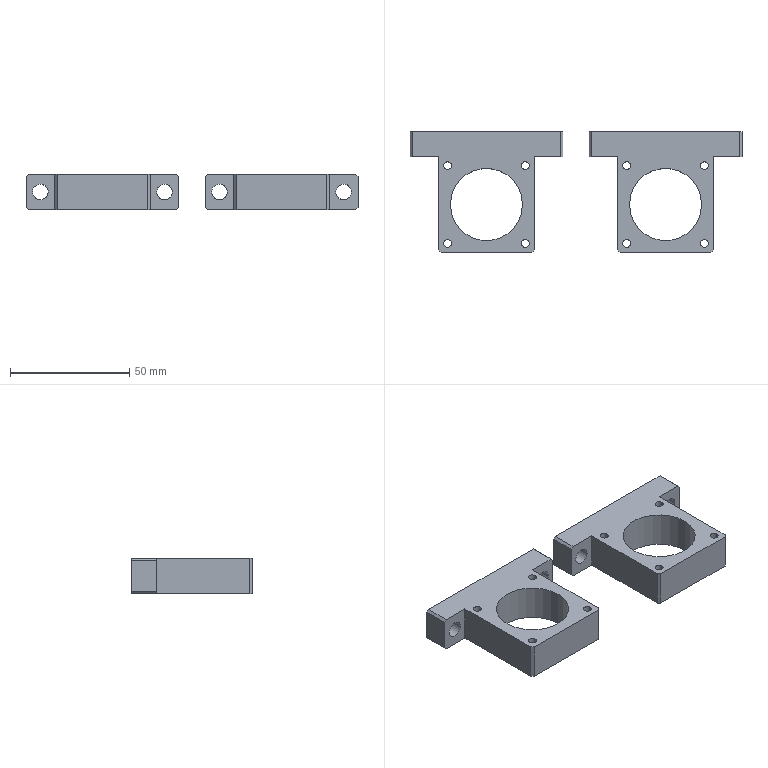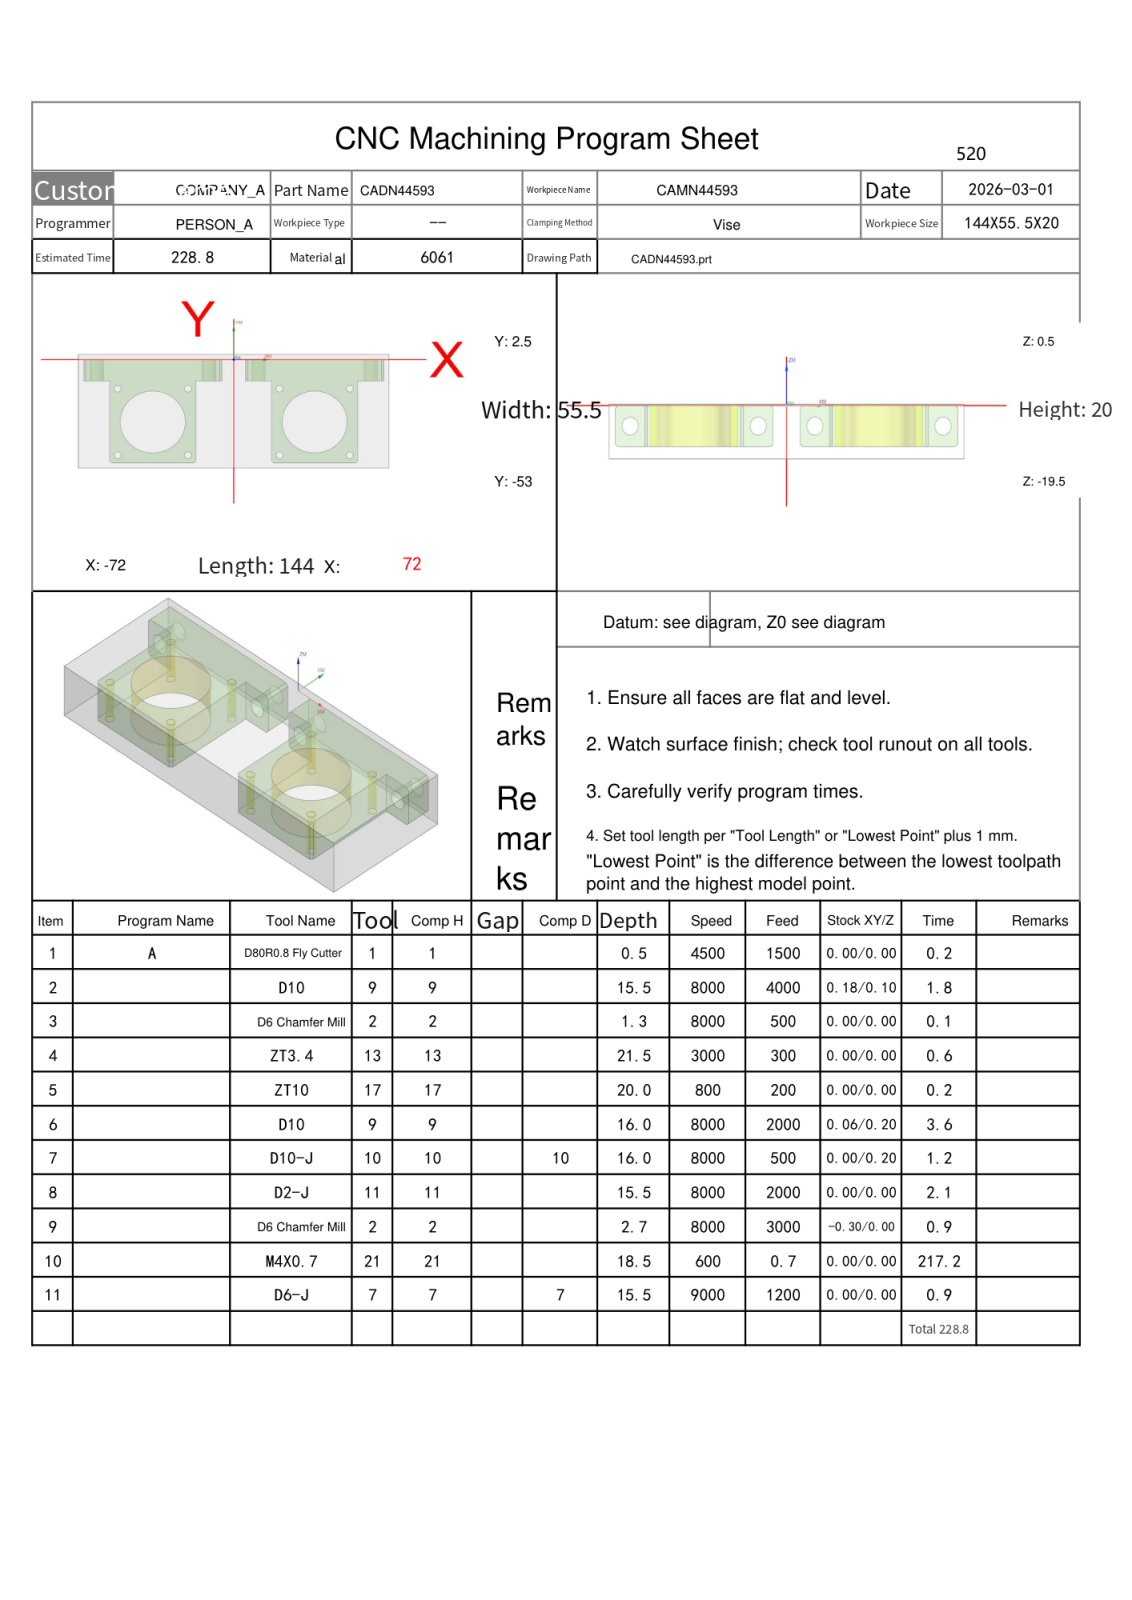NC program | NX | posted by the shop | part box 139 x 50.5 x 15 mm
Lines 36 to 892 of 10033:
N2 T09 M06
(D10  D=10. R=0. H=09 ce=0.25 di=0.10)
G00 G90 G54 X-82.431 Y-11.514 M03 S8000
G43 H09 Z50.
M08
Z-13.
G01 X-82.332 Y-11.496 Z-13.625 F4000.
X-82.234 Y-11.477 Z-13.872
X-82.136 Y-11.458 Z-14.054
X-82.038 Y-11.44 Z-14.2
X-81.939 Y-11.421 Z-14.323
X-81.841 Y-11.402 Z-14.428
X-81.743 Y-11.384 Z-14.52
X-81.645 Y-11.365 Z-14.6
X-81.546 Y-11.346 Z-14.67
X-81.448 Y-11.328 Z-14.732
X-81.35 Y-11.309 Z-14.786
X-81.252 Y-11.29 Z-14.833
X-81.153 Y-11.272 Z-14.874
X-81.055 Y-11.253 Z-14.908
X-80.957 Y-11.234 Z-14.936
X-80.859 Y-11.216 Z-14.96
X-80.761 Y-11.197 Z-14.977
X-80.662 Y-11.178 Z-14.99
X-80.564 Y-11.16 Z-14.997
X-80.466 Y-11.141 Z-15.
X-78.352 Y-10.739
G03 X-78. Y-10.48 I-.101 J.505
X-77.362 Y-6.666 I-12.273 J4.014
X-77.171 Y.847 I-456.093 J15.32
G02 X-73.96 Y5.724 I6.172 J-.569
X-68.324 Y7.378 I6.632 J-12.167
X-60.544 Y7.699 I7.779 J-93.942
X-59.293 Y7.691 I0.0 J-94.264
G01 X70.13 Y7.678
G02 X75.219 Y4.452 I-.351 J-6.181
X76.887 Y-1.277 I-12.247 J-6.672
X77.2 Y-9.063 I-96.712 J-7.786
X77.192 Y-10.308 I-97.025 J0.0
G01 X77.178 Y-51.13
G02 X73.969 Y-56.209 I-6.178 J.35
X68.412 Y-57.866 I-6.606 J12.012
X60.704 Y-58.198 I-7.708 J89.284
X59.542 Y-58.19 I0.0 J89.616
G01 X-70.15 Y-58.176
G02 X-75.222 Y-54.947 I.374 J6.185
X-76.868 Y-49.389 I12.074 J6.599
X-77.206 Y-41.288 I97.034 J8.1
X-77.193 Y-39.718 I97.372 J0.0
G01 X-77.183 Y-13.259
G03 X-76.595 Y-6.386 I-443.932 J41.454
G02 X-76.388 Y-1.091 I468.298 J-15.653
X-72.222 Y4.757 I7.74 J-1.105
X-65.87 Y6.544 I7.573 J-14.737
X-57.126 Y6.901 I8.744 J-106.812
X-55.64 Y6.891 I0.0 J-107.17
G01 X67.987 Y6.879
G02 X74.202 Y2.785 I-.602 J-7.679
X76.033 Y-3.55 I-14.344 J-7.577
X76.402 Y-12.347 I-104.524 J-8.797
X76.391 Y-13.859 I-104.894 J0.0
G01 X76.379 Y-48.987
G02 X72.413 Y-55.125 I-7.648 J.591
X66.168 Y-57.003 I-7.584 J13.897
X57.695 Y-57.396 I-8.473 J91.309
X56.5 Y-57.388 I0.0 J91.702
G01 X-67.987 Y-57.379
G02 X-74.125 Y-53.413 I.591 J7.648
X-76.003 Y-47.168 I13.895 J7.585
X-76.395 Y-38.7 I91.242 J8.468
X-76.388 Y-37.5 I91.635 J0.0
G01 X-76.379 Y-14.881
G02 X-75.807 Y-6.094 I948.959 J-57.37
X-75.532 Y-2.233 I27.725 J-.031
X-74.749 Y.011 I10.239 J-2.318
G01 X-74.571 Y1.359
X-74.047 Y2.625
X-73.212 Y3.712
X-72.125 Y4.547
X-70.859 Y5.071
G02 X-57.018 Y6.08 I13.841 J-94.414
X-56.024 Y6.075 I0.0 J-95.423
G01 X65.955 Y6.076
G02 X69.277 Y5.268 I-.437 J-9.032
G01 X70.859 Y5.071
X72.125 Y4.547
X73.212 Y3.712
X74.047 Y2.625
X74.571 Y1.359
G02 X75.577 Y-12.39 I-93.437 J-13.748
G01 X75.576 Y-12.82
X75.575 Y-46.959
G02 X70.823 Y-54.292 I-8.747 J.463
X64.171 Y-56.187 I-8.15 J15.986
X54.605 Y-56.608 I-9.566 J108.501
X52.744 Y-56.592 I0.0 J108.921
G01 X-65.956 Y-56.575
G02 X-73.291 Y-51.823 I.46 J8.748
X-75.177 Y-45.251 I15.886 J8.116
X-75.593 Y-36.287 I96.443 J8.963
X-75.586 Y-35.104 I96.859 J0.0
X-75.621 Y-26.982 I943.081 J8.122
X-75.546 Y-15.125 I943.116 J0.0
X-74.908 Y-4.653 I566.659 J-29.296
G01 X-74.75 Y-3.687
X-74.739 Y.081
G02 X-74.733 Y-2.973 I-765.948 J-3.054
X-74.784 Y-11.75 I-765.954 J0.0
G03 X-74.978 Y-23.864 I376.811 J-12.114
X-74.958 Y-27.735 I377.006 J0.0
X-74.977 Y-30.988 I290.447 J-3.254
X-74.769 Y-41.972 I290.465 J0.0
X-73.565 Y-49.046 I25.763 J.744
X-66.385 Y-55.337 I8.769 J2.765
X-59.903 Y-55.919 I6.482 J35.854
X-59.54 Y-55.917 I0.0 J36.435
G01 X-48.821 Y-55.958
X55.639 Y-55.931
G03 X56.143 Y-55.933 I.504 J68.081
X64.577 Y-55.409 I0.0 J68.083
X70.57 Y-53.308 I-1.709 J14.474
X74.323 Y-47.452 I-5.219 J7.475
X74.925 Y-40.804 I-36.403 J6.648
X74.921 Y-40.289 I-37.005 J0.0
G01 X74.958 Y-21.509
G03 X74.974 Y-18.479 I-302.812 J3.03
X74.75 Y-6.843 I-302.827 J0.0
G01 Y-.002
Y-10.502
G03 X74.175 Y-18.196 I51.208 J-7.694
X74.182 Y-19.024 I51.783 J0.0
G01 X74.119 Y-39.688
G02 X74.121 Y-40.113 I-33.926 J-.425
X73.539 Y-46.371 I-33.929 J0.0
X67.783 Y-53.21 I-9.493 J2.149
X60.803 Y-54.831 I-8.326 J20.008
G03 X59.177 Y-55.005 I.063 J-8.269
G02 X56.639 Y-55.748 I-2.829 J4.959
G01 X18.498 Y-55.75
G03 X10.852 Y-55.183 I-7.646 J-51.258
X10.208 Y-55.187 I0.0 J-51.826
G01 X-16.148 Y-55.171
X-17.141 Y-55.571
X-18.502 Y-55.75
X-56.642 Y-55.748
G03 X-63.405 Y-54.926 I-17.06 J-112.182
G02 X-68.664 Y-53.161 I.998 J11.687
X-72.813 Y-47.233 I6.532 J8.988
X-73.982 Y-39.664 I28.771 J8.321
X-74.182 Y-26.992 I402.551 J12.671
X-74.156 Y-22.466 I402.75 J0.0
X-74.05 Y-13.132 I612.773 J-2.32
G01 X-74.571 Y-11.859
X-74.75 Y-10.5
X-74.571 Y-11.859
G02 X-73.631 Y-15.867 I-8.072 J-4.008
G01 Y-15.908
G02 X-73.493 Y-26.765 I-426.487 J-10.858
X-73.51 Y-30.613 I-426.625 J0.0
G03 X-73.52 Y-32.179 I120.675 J-1.566
X-73.149 Y-41.643 I120.685 J0.0
X-71.428 Y-48.35 I19.187 J1.348
X-64.936 Y-53.583 I9.13 J4.683
X-59.767 Y-54.635 I11.418 J42.874
X-57.879 Y-55.57 I4.27 J6.245
G02 X-59.94 Y-54.497 I2.18 J6.698
G03 X-63.341 Y-53.256 I-10.094 J-22.38
G02 X-69.204 Y-49.355 I3.288 J11.298
X-71.958 Y-42.678 I12.418 J9.029
X-72.663 Y-33.723 I56.485 J8.955
G01 Y-33.515
X-72.775 Y-18.171
Y-18.061
G03 X-73.149 Y-14.317 I-18.885 J0.0
G01 X-74.047 Y-13.125
G02 X-72.957 Y-14.636 I-7.181 J-6.325
X-72.241 Y-18.739 I-12.6 J-4.313
X-72.046 Y-29.331 I-287.569 J-10.592
X-72.051 Y-31.028 I-287.764 J0.0
G03 X-72.056 Y-31.857 I74.824 J-.83
X-71.475 Y-41.163 I74.828 J0.0
X-69.154 Y-47.762 I16.108 J1.957
X-63.631 Y-52.166 I10.343 J7.308
G02 X-61.112 Y-53.319 I-20.619 J-48.377
G03 X-59.669 Y-54.684 I28.432 J28.599
G02 X-61.112 Y-53.319 I10.189 J12.211
G03 X-63.344 Y-51.644 I-7.49 J-7.657
G02 X-68.751 Y-46.08 I7.259 J12.463
X-70.803 Y-38.723 I18.983 J9.261
X-71.27 Y-28.82 I104.897 J9.903
X-71.265 Y-27.778 I105.364 J0.0
G03 X-71.256 Y-26.385 I-114.303 J1.393
X-71.552 Y-18.17 I-114.312 J0.0
X-72.325 Y-14.916 I-9.237 J-.477
G01 X-73.212 Y-14.212
G02 X-72.137 Y-15.11 I-2.708 J-4.339
X-71.08 Y-18.419 I-7.003 J-4.061
X-70.656 Y-25.71 I-62.477 J-7.291
G01 Y-25.957
X-70.657 Y-26.409
G03 X-70.267 Y-37.215 I149.848 J0.0
X-68.421 Y-44.795 I22.579 J1.482
X-63.647 Y-50.425 I13.848 J6.904
G02 X-62.356 Y-51.504 I-5.852 J-8.313
G03 X-61.225 Y-53.196 I5.165 J2.23
G02 X-62.473 Y-51.245 I4.692 J4.377
G03 X-64.739 Y-48.532 I-23.525 J-17.349
G02 X-69.063 Y-38.943 I14.543 J12.327
X-69.794 Y-28.991 I67.41 J9.952
G01 Y-28.979
Y-28.838
G03 X-70.193 Y-19.713 I-104.458 J0.0
X-71.268 Y-15.662 I-11.361 J-.847
X-72.125 Y-15.047 I-1.109 J-.64
G01 X-72.379 Y-14.852
G03 X-71.53 Y-15.293 I1.458 J1.768
G02 X-70.22 Y-17.527 I-3.011 J-3.268
X-69.36 Y-23.349 I-23.843 J-6.496
G03 X-68.953 Y-33.765 I924.383 J30.898
X-67.431 Y-42.243 I31.323 J1.249
X-63.91 Y-48.305 I19.584 J7.322
G02 X-62.711 Y-49.98 I-10.07 J-8.467
G03 X-62.344 Y-51.499 I4.612 J.312
G02 X-62.758 Y-49.691 I6.886 J2.53
G03 X-64.405 Y-46.484 I-17.564 J-6.992
G02 X-67.928 Y-35.183 I23.689 J13.585
X-68.496 Y-24.9 I170.445 J14.57
G03 X-69.37 Y-18.191 I-30.901 J-.615
X-70.631 Y-15.67 I-5.904 J-1.377
G01 X-71.598 Y-15.265
G02 X-70.51 Y-15.718 I-2.748 J-8.132
X-68.968 Y-18.253 I-3.654 J-3.959
X-67.945 Y-24.45 I-24.694 J-7.259
G03 X-67.341 Y-34.242 I316.925 J14.627
X-63.573 Y-46.518 I29.872 J2.452
G02 X-62.75 Y-48.355 I-12.898 J-6.884
G01 X-62.751 Y-48.562
G03 X-62.708 Y-49.917 I21.649 J0.0
G02 X-62.762 Y-47.989 I34.497 J1.928
G01 Y-47.948
G03 X-63.736 Y-44.797 I-14.136 J-2.643
G02 X-66.704 Y-31.486 I37.919 J15.44
G03 X-67.39 Y-22.37 I-180.615 J-9.014
X-68.834 Y-17.111 I-15.436 J-1.412
X-70.058 Y-15.686 I-2.961 J-1.306
G01 X-70.859 Y-15.571
G02 X-69.766 Y-15.79 I-.065 J-3.162
X-67.969 Y-18.171 I-2.941 J-4.088
X-66.629 Y-24.212 I-19.916 J-7.587
G03 X-65.835 Y-33.62 I890.373 J70.394
X-63.21 Y-44.292 I43.374 J5.012
G01 X-62.75 Y-45.743
Y-48.143
G03 X-62.727 Y-46.823 I-37.301 J1.32
X-62.798 Y-44.518 I-37.325 J0.0
X-63.99 Y-39.239 I-75.218 J-14.218
G02 X-65.465 Y-28.379 I71.773 J15.276
G03 X-66.515 Y-20.531 I-49.341 J-2.608
X-68.472 Y-16.358 I-9.618 J-1.964
X-69.322 Y-15.75 I-1.342 J-.979
G01 X-70.057 Y-15.677
G02 X-68.974 Y-15.829 I-.159 J-5.043
X-66.967 Y-18.096 I-2.488 J-4.224
X-65.33 Y-24.057 I-17.553 J-8.026
X-64.328 Y-33.318 I-746.439 J-85.447
G03 X-62.75 Y-41.617 I79.908 J10.89
G01 Y-45.057
G03 X-62.727 Y-42.921 I-100.07 J2.136
X-62.798 Y-39.166 I-100.093 J0.0
G02 X-64.402 Y-25.217 I930.073 J114.005
G03 X-66.051 Y-18.619 I-23.568 J-2.389
X-68.259 Y-15.82 I-5.837 J-2.331
X-68.975 Y-15.732 I-.716 J-2.882
X-69.298 Y-15.75 I0.0 J-2.97
G02 X-68.929 Y-15.73 I.369 J-3.387
X-68.13 Y-15.825 I0.0 J-3.407
X-65.914 Y-18.081 I-2.318 J-4.493
X-64.012 Y-24.113 I-16.691 J-8.582
X-62.824 Y-33.58 I-234.805 J-34.266
G01 X-62.75 Y-34.171
Y-40.011
G03 X-62.739 Y-36.028 I-708.891 J3.983
X-62.779 Y-28.511 I-708.902 J0.0
X-64.494 Y-19.645 I-29.831 J-1.172
X-66.966 Y-16.055 I-7.736 J-2.68
X-67.56 Y-15.75 I-1.118 J-1.447
G01 X-68.44
G02 X-68.018 Y-15.727 I.421 J-3.884
X-67.213 Y-15.811 I0.0 J-3.907
X-64.881 Y-17.997 I-2.176 J-4.658
X-62.75 Y-24.115 I-15.397 J-8.793
G01 Y-29.155
G03 X-62.726 Y-26.477 I-150.841 J2.679
X-62.785 Y-22.27 I-150.865 J0.0
X-65.484 Y-16.445 I-9.71 J-.96
X-66.568 Y-15.75 I-1.9 J-1.772
G01 X-67.528
G02 X-67.1 Y-15.731 I.427 J-4.891
X-66.206 Y-15.813 I0.0 J-4.91
X-63.838 Y-17.991 I-2.135 J-4.7
X-62.75 Y-20.414 I-8.344 J-5.201
G01 Y-22.814
G03 X-62.725 Y-21.613 I-28.936 J1.201
X-62.794 Y-19.623 I-28.961 J0.0
X-65.435 Y-15.784 I-5.498 J-.955
X-66.285 Y-15.746 I-.85 J-9.4
X-66.556 Y-15.75 I0.0 J-9.439
G02 X-66.12 Y-15.729 I.436 J-4.585
X-65.226 Y-15.817 I0.0 J-4.606
X-62.75 Y-18.632 I-1.899 J-4.166
G01 Y-20.072
G03 X-62.725 Y-19.377 I-9.686 J.696
X-62.821 Y-18.017 I-9.711 J0.0
X-64.64 Y-15.769 I-3.473 J-.949
G01 X-65.54 Y-15.75
G02 X-65.146 Y-15.726 I.393 J-3.224
X-64.389 Y-15.815 I0.0 J-3.248
X-62.75 Y-17.578 I-1.154 J-2.717
G01 Y-18.458
G03 X-62.729 Y-18.03 I-4.319 J.428
X-62.839 Y-17.06 I-4.341 J0.0
X-64.009 Y-15.764 I-2.105 J-.725
G01 X-64.736 Y-15.75
G02 X-64.407 Y-15.726 I.329 J-2.23
X-63.744 Y-15.825 I0.0 J-2.254
X-62.75 Y-16.943 I-.72 J-1.642
G01 Y-17.423
G03 X-62.727 Y-17.155 I-1.577 J.268
X-63.501 Y-15.785 I-1.6 J0.0
G01 X-64.062 Y-15.75
G02 X-63.84 Y-15.728 I.222 J-1.109
X-62.75 Y-16.558 I0.0 J-1.131
G01 Y-16.878
G03 X-62.727 Y-16.664 I-.983 J.214
X-63.281 Y-15.765 I-1.006 J0.0
G01 X-63.596 Y-15.75
X-63.477 Y-15.741
G02 X-62.842 Y-16.087 I0.0 J-.755
X-62.756 Y-16.382 I-.464 J-.295
X-63.306 Y-16.932 I-.55 J0.0
X-63.682 Y-16.784 I0.0 J.55
X-63.934 Y-16.312 I.316 J.472
X-63.628 Y-15.809 I.568 J0.0
X-63.37 Y-15.754 I.258 J-.578
X-62.737 Y-16.387 I0.0 J-.633
G01 X-62.75 Y-16.516
G02 X-63.021 Y-16.961 I-.504 J.003
G01 X-63.701 Y-17.31
X-65.454 Y-18.211 Z-14.9
X-66.363 Y-18.679
X-66.436 Y-18.709
X-66.513 Y-18.728
X-66.592 Y-18.734
X-72.807
X-72.987 Y-18.727
X-73.166 Y-18.705
X-73.343 Y-18.668
X-73.516 Y-18.617
X-73.684 Y-18.552
X-73.846 Y-18.473
X-74.002 Y-18.382
X-74.149 Y-18.278
X-74.288 Y-18.162
X-74.416 Y-18.036
X-74.534 Y-17.899
X-74.64 Y-17.753
X-76.037 Y-15.658
X-76.226 Y-15.363
X-76.407 Y-15.063
X-76.577 Y-14.756
X-76.738 Y-14.445
X-76.889 Y-14.128
X-77.029 Y-13.807
X-77.159 Y-13.481
X-77.277 Y-13.152
X-77.382 Y-12.818
X-77.473 Y-12.481
X-77.551 Y-12.14
X-77.615 Y-11.796
X-77.665 Y-11.45
X-77.701 Y-11.102
X-78.104 Y-6.265
X-78.149 Y-5.642
X-78.179 Y-5.018
X-78.194 Y-4.394
Y-3.769
X-78.18 Y-3.145
X-78.151 Y-2.521
X-78.107 Y-1.898
X-78.048 Y-1.276
X-77.975 Y-.656
X-77.887 Y-.038
X-77.784 Y.578
X-77.667 Y1.192
X-77.228 Y3.352
X-77.176 Y3.576
X-77.111 Y3.797
X-77.034 Y4.013
X-76.944 Y4.225
X-76.842 Y4.431
X-76.729 Y4.631
X-76.604 Y4.825
X-76.468 Y5.01
X-76.322 Y5.188
X-76.166 Y5.357
X-76.001 Y5.517
X-75.827 Y5.667
X-75.644 Y5.807
X-73.34 Y7.468
X-73.274 Y7.509
X-73.202 Y7.538
X-73.126 Y7.556
X-73.049 Y7.563
X-72.971 Y7.557
X-72.895 Y7.539
X-72.823 Y7.509
X-72.757 Y7.469
X-72.327 Y7.162
X-70.724 Y6.013 Z-15.
X-69.723 Y5.303
X-69.498 Y5.25
X-3.682 Y5.274
X63.749 Y5.287
G03 X67.5 Y5.236 I3.751 J136.982
X69.45 Y5.25 I0.0 J137.033
G01 X5.502
G02 X-1.944 Y4.665 I-7.445 J47.061
X-3.2 Y4.681 I0.0 J47.647
G01 X-4.141 Y5.071
X-5.498 Y5.25
X-4.141 Y5.071
G03 X-.041 Y4.14 I4.1 J8.558
X.202 Y4.143 I0.0 J9.49
X.922 Y4.115 I.72 J9.324
X2.452 Y4.241 I0.0 J9.352
G01 X2.875 Y4.547
X4.141 Y5.071
X2.875 Y4.547
G02 X1.087 Y3.849 I-1.905 J2.242
X-.208 Y3.742 I-1.295 J7.825
X-2.122 Y3.977 I0.0 J7.931
G01 X-2.949 Y4.577
G03 X-1.672 Y3.717 I5.43 J6.681
X.221 Y3.347 I1.893 J4.657
X1.607 Y3.542 I0.0 J5.027
G01 X2.486 Y4.248
G03 X1.637 Y3.532 I2.168 J-3.431
G02 X-.094 Y3.113 I-1.731 J3.368
X-1.488 Y3.379 I0.0 J3.787
G03 X-2.042 Y3.907 I-4.04 J-3.681
G02 X-1.514 Y3.362 I-1.305 J-1.791
G03 X.119 Y2.834 I1.633 J2.264
X1.29 Y3.092 I0.0 J2.792
G01 X1.702 Y3.601
G02 X.154 Y2.674 I-1.549 J.829
G01 X.073 Y2.675
G02 X-.131 Y2.665 I-.204 J1.963
X-1.252 Y3.014 I0.0 J1.973
G01 X-1.593 Y3.459
G03 X.102 Y2.452 I1.695 J.924
X.925 Y2.636 I0.0 J1.93
G01 X1.322 Y3.105
G02 X.04 Y2.323 I-1.282 J.659
X-.294 Y2.362 I0.0 J1.441
X-1.25 Y3.011 I.115 J1.197
G03 X.098 Y2.194 I1.347 J.703
X.73 Y2.332 I0.0 J1.52
G01 X1.002 Y2.688
G02 X.07 Y2.078 I-.932 J.405
X-.144 Y2.1 I0.0 J1.016
G01 X-.17
G02 X-.953 Y2.625 I0.0 J.847
G03 X.001 Y1.955 I.954 J.344
X.216 Y1.978 I0.0 J1.014
X.923 Y2.551 I-.014 J.739
G02 X.036 Y1.875 I-.886 J.244
X-.245 Y1.919 I0.0 J.92
X-.874 Y2.435 I.082 J.742
G03 X.014 Y1.773 I.889 J.267
X.751 Y2.136 I0.0 J.928
G01 X.843 Y2.358
G02 X-.009 Y1.706 I-.851 J.229
X-.414 Y1.804 I0.0 J.882
X-.791 Y2.234 I.316 J.658
G03 X.007 Y1.625 I.798 J.218
X.686 Y1.98 I0.0 J.828
G01 X.778 Y2.202
G02 X.008 Y1.568 I-.77 J.151
X-.723 Y2.069 I0.0 J.785
G03 X-.005 Y1.495 I.718 J.161
X.658 Y1.911 I0.0 J.736
G02 X0.0 Y1.443 I-.657 J.228
X-.634 Y1.853 I0.0 J.696
G03 X-.001 Y1.383 I.632 J.19
X.622 Y1.825 I0.0 J.66
G02 X.004 Y1.341 I-.618 J.153
X-.577 Y1.716 I0.0 J.637
G03 X-.001 Y1.285 I.576 J.169
X.569 Y1.698 I0.0 J.6
G02 X0.0 Y1.211 I-.569 J.09
X-.569 Y1.698 I0.0 J.576
G01 X-.601 Y1.973
G02 X-.022 Y5.32 I165.225 J-26.846
G01 X.067 Y5.447
X.138 Y5.518 Z-14.997
X.209 Y5.589 Z-14.99
X.279 Y5.66 Z-14.977
X.35 Y5.73 Z-14.96
X.421 Y5.801 Z-14.936
X.491 Y5.872 Z-14.908
X.562 Y5.942 Z-14.874
X.633 Y6.013 Z-14.833
X.704 Y6.084 Z-14.786
X.774 Y6.155 Z-14.732
X.845 Y6.225 Z-14.67
X.916 Y6.296 Z-14.6
X.986 Y6.367 Z-14.52
X1.057 Y6.437 Z-14.428
X1.128 Y6.508 Z-14.323
X1.199 Y6.579 Z-14.2
X1.269 Y6.65 Z-14.054
X1.34 Y6.72 Z-13.872
X1.411 Y6.791 Z-13.625
X1.481 Y6.862 Z-13.
G00 Z50.
X16.373 Y-59.675
Z-13.
G01 X16.436 Y-59.597 Z-13.625
X16.499 Y-59.52 Z-13.872
X16.562 Y-59.442 Z-14.054
X16.625 Y-59.364 Z-14.2
X16.688 Y-59.287 Z-14.323
X16.751 Y-59.209 Z-14.428
X16.814 Y-59.131 Z-14.52
X16.877 Y-59.054 Z-14.6
X16.94 Y-58.976 Z-14.67
X17.003 Y-58.898 Z-14.732
X17.066 Y-58.821 Z-14.786
X17.129 Y-58.743 Z-14.833
X17.192 Y-58.665 Z-14.874
X17.255 Y-58.588 Z-14.908
X17.318 Y-58.51 Z-14.936
X17.381 Y-58.432 Z-14.96
X17.444 Y-58.355 Z-14.977
X17.508 Y-58.277 Z-14.99
X17.571 Y-58.199 Z-14.997
X17.634 Y-58.122 Z-15.
G03 X17.746 Y-57.8 I-.406 J.322
G01 X17.74 Y-57.721
X17.446 Y-55.955
G03 X17.141 Y-55.571 I-.503 J-.087
X12.979 Y-54.623 I-4.661 J-10.855
X3.812 Y-54.345 I-9.167 J-150.817
X1.691 Y-54.36 I0.0 J-151.095
X-4.703 Y-54.337 I-6.393 J-916.734
X-14.607 Y-54.391 I0.0 J-916.756
X-15.177 Y-54.511 I.103 J-1.905
G02 X-16.245 Y-55.2 I-2.339 J2.454
G03 X-15.113 Y-54.462 I-1.406 J3.393
G02 X-12.339 Y-53.909 I2.914 J-7.377
X-3.635 Y-53.701 I8.704 J-181.964
X-1.112 Y-53.718 I0.0 J-182.172
X1.736 Y-53.699 I2.847 J-214.021
X11.792 Y-53.935 I0.0 J-214.04
X15.006 Y-54.391 I-1.021 J-18.761
G01 X15.875 Y-55.047
X16.392 Y-55.261
G02 X15.052 Y-54.415 I1.419 J3.733
G03 X12.213 Y-53.448 I-3.502 J-5.626
X4.795 Y-52.956 I-7.418 J-55.688
X4.356 Y-52.958 I0.0 J-56.18
X-1.296 Y-52.898 I-5.652 J-267.15
X-11.083 Y-53.077 I0.0 J-267.21
X-14.098 Y-53.553 I.386 J-12.241
G02 X-15.17 Y-54.506 I-10.845 J11.121
G03 X-14.072 Y-53.505 I-6.103 J7.805
G02 X-11.063 Y-52.639 I3.563 J-6.718
X-3.507 Y-52.282 I7.556 J-79.628
X-2.216 Y-52.292 I0.0 J-79.985
X.395 Y-52.269 I2.611 J-145.567
X9.797 Y-52.573 I0.0 J-145.591
X13.971 Y-53.419 I-.812 J-14.718
G01 X14.977 Y-54.357
X13.799 Y-53.247
G03 X10.435 Y-52.078 I-4.356 J-7.111
X2.445 Y-51.523 I-7.99 J-57.23
X1.977 Y-51.525 I0.0 J-57.785
X-1.379 Y-51.479 I-3.356 J-122.333
X-9.605 Y-51.756 I0.0 J-122.379
X-13.187 Y-52.532 I.691 J-11.837
G01 X-14.184 Y-53.609
G03 X-13.206 Y-52.52 I-20.31 J19.236
G02 X-10.317 Y-51.419 I3.709 J-5.396
X-3.134 Y-50.887 I7.183 J-48.194
X-2.503 Y-50.891 I0.0 J-48.726
X-.033 Y-50.859 I2.47 J-94.596
X8.796 Y-51.272 I0.0 J-94.628
X13.046 Y-52.368 I-1.08 J-12.973
G01 X13.957 Y-53.381
G03 X12.837 Y-52.117 I-15.691 J-12.773
X9.234 Y-50.758 I-4.81 J-7.296
X1.12 Y-50.118 I-8.114 J-51.103
X.679 Y-50.12 I0.0 J-51.743
X-1.419 Y-50.088 I-2.098 J-69.532
X-8.891 Y-50.491 I0.0 J-69.564
X-12.612 Y-51.594 I.939 J-10.
X-13.206 Y-52.52 I2.818 J-2.459
G02 X-12.421 Y-51.371 I3.495 J-1.543
X-8.962 Y-50.053 I4.516 J-6.655
X-1.512 Y-49.489 I7.451 J-48.914
X-.396 Y-49.501 I0.0 J-49.478
X.661 Y-49.49 I1.057 J-52.228
X8.928 Y-50.149 I0.0 J-52.239
X12.57 Y-51.497 I-1.436 J-9.474
X13.19 Y-52.493 I-5.297 J-3.987
G03 X12.433 Y-51.256 I-6.143 J-2.906
X9.277 Y-49.687 I-4.665 J-5.425
X1.566 Y-48.782 I-7.889 J-33.922
X-.925 Y-48.723 I-2.491 J-53.088
X-8.212 Y-49.225 I0.0 J-53.147
X-12.117 Y-50.601 I1.186 J-9.596
X-12.486 Y-50.98 I1.045 J-1.386
G01 X-12.75 Y-51.736
G02 X-12.299 Y-50.657 I3.624 J-.882
X-9.536 Y-49.105 I4.167 J-4.186
X-2.412 Y-48.184 I7.153 J-27.291
X-.181 Y-48.132 I2.231 J-47.877
X7.862 Y-48.812 I0.0 J-47.929
X11.901 Y-50.359 I-1.679 J-10.425
X12.457 Y-50.898 I-1.466 J-2.067
G01 X12.721 Y-51.654
G03 X10.879 Y-49.359 I-3.237 J-.712
X5.772 Y-47.83 I-6.715 J-13.131
X-.494 Y-47.395 I-6.267 J-44.96
X-7.518 Y-47.942 I0.0 J-45.395
X-11.684 Y-49.523 I1.476 J-10.168
X-12.33 Y-50.258 I.8 J-1.355
G02 X-12.482 Y-50.969 I-2.618 J.186
G03 X-12.302 Y-50.101 I-3.432 J1.164
G02 X-10.284 Y-48.386 I3.556 J-2.141
X-4.518 Y-47.021 I6.806 J-15.886
X-.435 Y-46.817 I4.083 J-40.682
X7.377 Y-47.57 I0.0 J-40.887
X11.627 Y-49.395 I-1.877 J-10.235
X12.328 Y-50.24 I-1.172 J-1.685
G03 X12.455 Y-50.894 I3.113 J.266
G02 X12.305 Y-50.082 I3.754 J1.117
G03 X10.579 Y-48.264 I-3.538 J-1.631
X5.243 Y-46.539 I-7.124 J-12.924
X-.437 Y-46.1 I-5.68 J-36.504
X-7.326 Y-46.748 I0.0 J-36.943
X-11.516 Y-48.555 I1.763 J-9.849
X-12.25 Y-49.499 I.964 J-1.507
G01 X-12.322 Y-50.182
G02 X-12.169 Y-49.152 I3.693 J-.021
X-9.818 Y-47.153 I4.212 J-2.572
X-3.387 Y-45.673 I7.282 J-16.929
X-.348 Y-45.534 I3.039 J-33.184
X7.457 Y-46.461 I0.0 J-33.323
X11.512 Y-48.472 I-2.256 J-9.642
X12.25 Y-49.499 I-1.336 J-1.738
G01 X12.321 Y-50.179
X12.322 Y-50.159
G03 X12.039 Y-48.812 I-3.347 J0.0
X9.286 Y-46.569 I-5.057 J-3.396
X2.166 Y-44.954 I-8.072 J-19.076
X-.541 Y-44.831 I-2.707 J-29.677
X-7.583 Y-45.675 I0.0 J-29.8
X-11.614 Y-47.752 I2.1 J-9.023
X-12.25 Y-48.695 I1.295 J-1.56
G01 Y-49.495
G02 X-12.27 Y-49.129 I3.425 J.366
X-12.178 Y-48.34 I3.444 J0.0
X-10.036 Y-46.234 I4.276 J-2.208
X-3.882 Y-44.488 I7.421 J-14.431
X-.365 Y-44.276 I3.517 J-29.124
X7.428 Y-45.33 I0.0 J-29.336
X11.569 Y-47.648 I-2.467 J-9.264
X12.25 Y-48.733 I-1.839 J-1.911
G01 Y-49.453
G03 X12.274 Y-49.085 I-2.801 J.368
X11.292 Y-46.943 I-2.825 J0.0
X6.738 Y-44.525 I-7.032 J-7.743
X-.397 Y-43.586 I-7.135 J-26.644
X-7.418 Y-44.494 I0.0 J-27.583
X-11.577 Y-46.761 I2.363 J-9.284
X-12.25 Y-47.79 I1.536 J-1.74
G01 Y-48.67
G02 X-12.268 Y-48.275 I4.342 J.395
X-12.187 Y-47.437 I4.36 J0.0
X-10.007 Y-45.165 I4.506 J-2.142
X-3.625 Y-43.246 I7.689 J-14.001
X-.338 Y-43.04 I3.287 J-26.128
X7.551 Y-44.25 I0.0 J-26.334
X11.69 Y-46.849 I-2.667 J-8.842
X12.25 Y-47.831 I-2.116 J-1.857
G01 Y-48.711
G03 X12.275 Y-48.28 I-3.761 J.431
X12.098 Y-47.136 I-3.786 J0.0
X9.414 Y-44.513 I-5.433 J-2.875
X2.304 Y-42.516 I-8.387 J-16.207
X-.467 Y-42.359 I-2.771 J-24.281
X-7.757 Y-43.471 I0.0 J-24.438
X-11.772 Y-45.981 I2.61 J-8.643
X-12.25 Y-46.814 I1.567 J-1.452
G01 Y-47.774
G02 X-12.27 Y-47.342 I4.757 J.432
X-12.185 Y-46.449 I4.776 J0.0
X-9.981 Y-44.076 I4.734 J-2.188
X-3.383 Y-42.016 I7.923 J-13.776
X-.314 Y-41.821 I3.069 J-24.095
X7.692 Y-43.179 I0.0 J-24.29
X11.671 Y-45.829 I-3.023 J-8.849
X12.25 Y-46.851 I-2.283 J-1.97
G01 Y-47.731
G03 X12.273 Y-47.3 I-3.955 J.431
X12.108 Y-46.163 I-3.979 J0.0
X9.405 Y-43.421 I-5.62 J-2.835
X2.074 Y-41.291 I-8.571 J-15.817
X-.466 Y-41.149 I-2.54 J-22.686
X-7.911 Y-42.397 I0.0 J-22.828
X-11.804 Y-44.992 I2.866 J-8.52
X-12.25 Y-45.791 I1.656 J-1.447
G01 Y-46.751
G02 X-12.274 Y-46.293 I4.46 J.458
X-12.192 Y-45.44 I4.483 J0.0
X-10.032 Y-43.018 I4.835 J-2.139
X-3.418 Y-40.828 I8.072 J-13.292
X-.309 Y-40.617 I3.109 J-22.783
X7.782 Y-42.087 I0.0 J-22.994
X11.734 Y-44.873 I-3.248 J-8.805
X12.25 Y-45.833 I-2.441 J-1.929
G01 Y-46.713
G03 X12.272 Y-46.282 I-4.213 J.431
X12.121 Y-45.16 I-4.235 J0.0
X9.463 Y-42.354 I-5.718 J-2.753
X1.987 Y-40.089 I-8.722 J-15.318
X-.462 Y-39.95 I-2.449 J-21.561
X-8.076 Y-41.33 I0.0 J-21.7
X-11.879 Y-44.03 I3.03 J-8.294
X-12.25 Y-44.745 I1.633 J-1.301
G01 Y-45.785
G02 X-12.27 Y-45.318 I5.498 J.467
X-12.189 Y-44.376 I5.517 J0.0
X-9.971 Y-41.871 I4.978 J-2.172
X-3.063 Y-39.6 I8.259 J-13.481
X-.287 Y-39.424 I2.776 J-21.812
X7.882 Y-40.998 I0.0 J-21.988
X11.855 Y-43.98 I-3.314 J-8.551
X12.25 Y-44.778 I-2.69 J-1.83
G01 Y-45.738
G03 X12.275 Y-45.269 I-4.388 J.469
X12.107 Y-44.063 I-4.413 J0.0
X9.478 Y-41.249 I-5.84 J-2.82
X1.77 Y-38.883 I-8.851 J-15.092
X-.473 Y-38.762 I-2.243 J-20.727
X-8.215 Y-40.253 I0.0 J-20.848
X-11.917 Y-43.001 I3.188 J-8.162
X-12.25 Y-43.652 I1.724 J-1.291
G01 Y-44.692
G02 X-12.269 Y-44.232 I5.488 J.46
X-12.188 Y-43.287 I5.507 J0.0
X-9.963 Y-40.748 I5.096 J-2.221
X-2.847 Y-38.396 I8.396 J-13.46
X-.266 Y-38.238 I2.581 J-21.041
X8.059 Y-39.941 I0.0 J-21.198
X11.89 Y-42.954 I-3.464 J-8.346
X12.25 Y-43.717 I-2.462 J-1.629
G01 Y-44.677
G03 X12.272 Y-44.213 I-4.824 J.464
X12.126 Y-43.031 I-4.846 J0.0
X9.507 Y-40.144 I-5.879 J-2.702
X1.826 Y-37.709 I-8.9 J-14.744
X-.465 Y-37.579 I-2.291 J-20.16
X-8.365 Y-39.18 I0.0 J-20.29
X-12.038 Y-42.08 I3.226 J-7.863
X-12.25 Y-42.553 I2.272 J-1.303
G01 Y-43.593
G02 X-12.269 Y-43.132 I5.55 J.461
X-12.188 Y-42.187 I5.569 J0.0
X-9.968 Y-39.624 I5.158 J-2.226
X-2.835 Y-37.219 I8.467 J-13.334
X-.268 Y-37.06 I2.567 J-20.649
X8.038 Y-38.79 I0.0 J-20.808
X11.901 Y-41.874 I-3.532 J-8.387
X12.25 Y-42.613 I-3.207 J-1.964
G01 Y-43.573
G03 X12.273 Y-43.109 I-4.768 J.464
X12.122 Y-41.917 I-4.79 J0.0
X9.487 Y-38.999 I-5.96 J-2.734
X1.551 Y-36.509 I-8.984 J-14.742
X-.487 Y-36.404 I-2.038 J-19.66
X-8.484 Y-38.094 I0.0 J-19.765
X-12.071 Y-41.021 I3.294 J-7.699
X-12.25 Y-41.441 I4.334 J-2.094
G01 Y-42.481
G02 X-12.27 Y-42.018 I5.468 J.462
X-12.187 Y-41.068 I5.487 J0.0
X-9.878 Y-38.428 I5.289 J-2.295
X-2.43 Y-36.006 I8.551 J-13.636
X-.234 Y-35.887 I2.196 J-20.152
X8.222 Y-37.735 I0.0 J-20.271
X11.92 Y-40.783 I-3.692 J-8.246
X12.25 Y-41.498 I-3.214 J-1.918
G01 Y-42.458
G03 X12.274 Y-41.987 I-4.712 J.471
X12.121 Y-40.796 I-4.736 J0.0
X9.524 Y-37.885 I-5.997 J-2.737
X1.413 Y-35.326 I-9.069 J-14.613
X-.501 Y-35.232 I-1.913 J-19.259
X-8.694 Y-37.052 I0.0 J-19.354
X-12.157 Y-40.044 I3.329 J-7.353
G01 X-12.25 Y-40.314
Y-41.434
G02 X-12.271 Y-40.936 I5.908 J.498
X-12.188 Y-39.945 I5.929 J0.0
X-10.005 Y-37.377 I5.233 J-2.237
X-2.753 Y-34.871 I8.589 J-13.113
X-.25 Y-34.715 I2.504 J-19.92
X8.278 Y-36.615 I0.0 J-20.077
X12.028 Y-39.843 I-3.623 J-8.004
G01 X12.25 Y-40.374
Y-41.414
G03 X12.274 Y-40.888 I-5.752 J.526
X12.18 Y-39.852 I-5.776 J0.0
X9.967 Y-37.06 I-5.546 J-2.122
X2.604 Y-34.288 I-9.113 J-13.046
X-.377 Y-34.064 I-2.981 J-19.677
X-8.23 Y-35.678 I0.0 J-19.902
X-11.966 Y-38.599 I3.485 J-8.309
X-12.25 Y-39.187 I1.958 J-1.306
G01 Y-40.307
G02 X-12.267 Y-39.824 I6.718 J.483
X-12.194 Y-38.834 I6.736 J0.0
X-10.015 Y-36.242 I5.224 J-2.181
X-2.617 Y-33.691 I8.648 J-13.077
X-.233 Y-33.547 I2.384 J-19.648
X8.402 Y-35.53 I0.0 J-19.792
X12.029 Y-38.713 I-3.714 J-7.892
G01 X12.25 Y-39.244
Y-40.284
G03 X12.275 Y-39.779 I-5.095 J.505
X12.124 Y-38.543 I-5.12 J0.0
X9.557 Y-35.618 I-6.045 J-2.717
X1.475 Y-32.998 I-9.111 J-14.328
X-.473 Y-32.898 I-1.948 J-19.047
X-8.636 Y-34.726 I0.0 J-19.146
X-12.072 Y-37.629 I3.526 J-7.656
G01 X-12.25 Y-38.05
Y-39.17
G02 X-12.274 Y-38.644 I5.71 J.526
X-12.196 Y-37.701 I5.734 J0.0
X-10.011 Y-35.091 I5.25 J-2.176
X-2.679 Y-32.534 I8.65 J-13.014
X-.24 Y-32.383 I2.439 J-19.581
X8.33 Y-34.341 I0.0 J-19.732
X12.032 Y-37.581 I-3.72 J-7.985